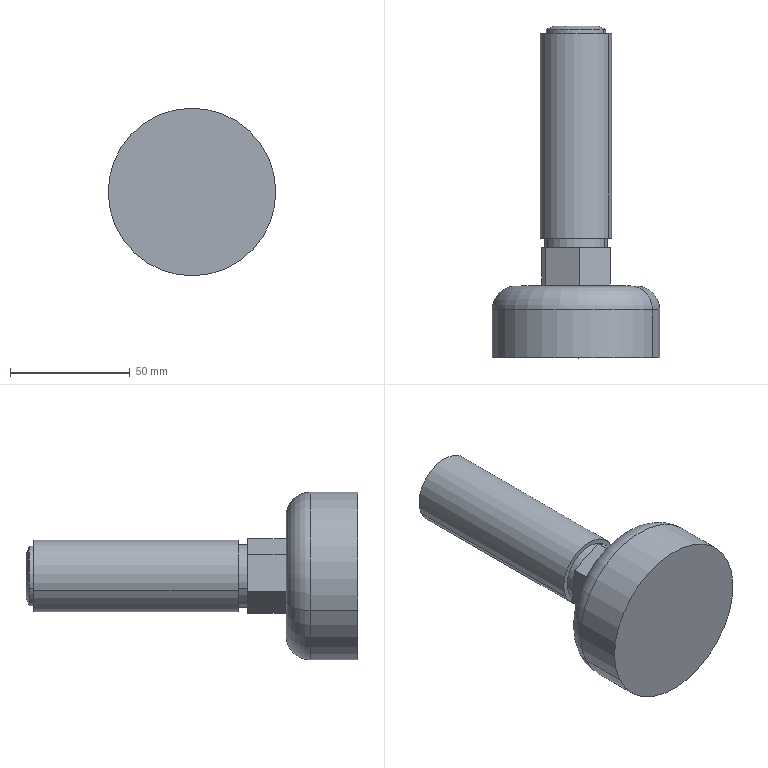Part | STEP file | Fillet 2-4 | 1 solid | 26 faces | box 70 x 138.618 x 70 mm | volume 157430 mm3 | plane 12 | cylinder 10 | torus 2 | sphere 2 | commonest cylinder face diameters 18 x2 25 x2 26 x2 30 x2 70 x2
STEP:
#1=CARTESIAN_POINT('',(-1171.526,-1356.736,3153.219));
#2=VERTEX_POINT('',#1);
#3=CARTESIAN_POINT('',(-1125.95,-1356.736,3173.781));
#4=VERTEX_POINT('',#3);
#5=CARTESIAN_POINT('',(-1148.738,-1356.736,3163.5));
#6=DIRECTION('',(0.,1.,0.));
#7=DIRECTION('',(0.9115,0.,0.4113));
#8=AXIS2_PLACEMENT_3D('',#5,#6,#7);
#9=CIRCLE('',#8,25.);
#10=EDGE_CURVE('',#2,#4,#9,.T.);
#11=ORIENTED_EDGE('',*,*,#10,.F.);
#12=CARTESIAN_POINT('',(-1180.641,-1366.736,3149.106));
#13=VERTEX_POINT('',#12);
#14=CARTESIAN_POINT('',(-1171.526,-1366.736,3153.219));
#15=DIRECTION('',(-0.4113,0.,0.9115));
#16=DIRECTION('',(-0.9115,0.,-0.4113));
#17=AXIS2_PLACEMENT_3D('',#14,#15,#16);
#18=CIRCLE('',#17,10.);
#19=EDGE_CURVE('',#2,#13,#18,.T.);
#20=ORIENTED_EDGE('',*,*,#19,.T.);
#21=CARTESIAN_POINT('',(-1116.835,-1366.736,3177.894));
#22=VERTEX_POINT('',#21);
#23=CARTESIAN_POINT('',(-1148.738,-1366.736,3163.5));
#24=DIRECTION('',(0.,-1.,0.));
#25=DIRECTION('',(0.9115,0.,0.4113));
#26=AXIS2_PLACEMENT_3D('',#23,#24,#25);
#27=CIRCLE('',#26,35.);
#28=EDGE_CURVE('',#22,#13,#27,.T.);
#29=ORIENTED_EDGE('',*,*,#28,.F.);
#30=CARTESIAN_POINT('',(-1125.95,-1366.736,3173.781));
#31=DIRECTION('',(0.4113,0.,-0.9115));
#32=DIRECTION('',(0.,1.,0.));
#33=AXIS2_PLACEMENT_3D('',#30,#31,#32);
#34=CIRCLE('',#33,10.);
#35=EDGE_CURVE('',#4,#22,#34,.T.);
#36=ORIENTED_EDGE('',*,*,#35,.F.);
#37=EDGE_LOOP('',(#11,#20,#29,#36));
#38=FACE_OUTER_BOUND('',#37,.T.);
#39=CARTESIAN_POINT('',(-1148.738,-1366.736,3163.5));
#40=DIRECTION('',(0.,-1.,0.));
#41=DIRECTION('',(-0.9115,0.,-0.4113));
#42=AXIS2_PLACEMENT_3D('',#39,#40,#41);
#43=TOROIDAL_SURFACE('',#42,25.,10.);
#44=ADVANCED_FACE('',(#38),#43,.T.);
#45=CARTESIAN_POINT('',(-1116.835,-1386.736,3177.894));
#46=VERTEX_POINT('',#45);
#47=CARTESIAN_POINT('',(-1180.641,-1386.736,3149.106));
#48=VERTEX_POINT('',#47);
#49=CARTESIAN_POINT('',(-1148.738,-1386.736,3163.5));
#50=DIRECTION('',(0.,-1.,0.));
#51=DIRECTION('',(0.9115,0.,0.4113));
#52=AXIS2_PLACEMENT_3D('',#49,#50,#51);
#53=CIRCLE('',#52,35.);
#54=EDGE_CURVE('',#46,#48,#53,.T.);
#55=ORIENTED_EDGE('',*,*,#54,.F.);
#56=CARTESIAN_POINT('',(-1116.835,-1386.736,3177.894));
#57=DIRECTION('',(0.,-1.,0.));
#58=VECTOR('',#57,1000.);
#59=LINE('',#56,#58);
#60=EDGE_CURVE('',#22,#46,#59,.T.);
#61=ORIENTED_EDGE('',*,*,#60,.F.);
#62=ORIENTED_EDGE('',*,*,#28,.T.);
#63=CARTESIAN_POINT('',(-1180.641,-1386.736,3149.106));
#64=DIRECTION('',(0.,-1.,0.));
#65=VECTOR('',#64,1000.);
#66=LINE('',#63,#65);
#67=EDGE_CURVE('',#13,#48,#66,.T.);
#68=ORIENTED_EDGE('',*,*,#67,.T.);
#69=EDGE_LOOP('',(#55,#61,#62,#68));
#70=FACE_OUTER_BOUND('',#69,.T.);
#71=CARTESIAN_POINT('',(-1148.738,-1386.736,3163.5));
#72=DIRECTION('',(0.,1.,0.));
#73=DIRECTION('',(0.9115,0.,0.4113));
#74=AXIS2_PLACEMENT_3D('',#71,#72,#73);
#75=CYLINDRICAL_SURFACE('',#74,35.);
#76=ADVANCED_FACE('',(#70),#75,.T.);
#77=CARTESIAN_POINT('',(-1160.132,-1251.236,3158.359));
#78=VERTEX_POINT('',#77);
#79=CARTESIAN_POINT('',(-1137.344,-1251.236,3168.641));
#80=VERTEX_POINT('',#79);
#81=CARTESIAN_POINT('',(-1148.738,-1251.236,3163.5));
#82=DIRECTION('',(0.,1.,0.));
#83=DIRECTION('',(-0.9115,0.,-0.4113));
#84=AXIS2_PLACEMENT_3D('',#81,#82,#83);
#85=CIRCLE('',#84,12.5);
#86=EDGE_CURVE('',#78,#80,#85,.T.);
#87=ORIENTED_EDGE('',*,*,#86,.T.);
#88=CARTESIAN_POINT('',(-1137.344,-1249.464,3168.641));
#89=VERTEX_POINT('',#88);
#90=CARTESIAN_POINT('',(-1137.344,-1246.736,3168.641));
#91=DIRECTION('',(0.,-1.,0.));
#92=VECTOR('',#91,1000.);
#93=LINE('',#90,#92);
#94=EDGE_CURVE('',#89,#80,#93,.T.);
#95=ORIENTED_EDGE('',*,*,#94,.F.);
#96=CARTESIAN_POINT('',(-1153.879,-1249.464,3174.894));
#97=VERTEX_POINT('',#96);
#98=CARTESIAN_POINT('',(-1148.738,-1249.464,3163.5));
#99=DIRECTION('',(0.,1.,0.));
#100=DIRECTION('',(-0.9115,0.,-0.4113));
#101=AXIS2_PLACEMENT_3D('',#98,#99,#100);
#102=CIRCLE('',#101,12.5);
#103=EDGE_CURVE('',#97,#89,#102,.T.);
#104=ORIENTED_EDGE('',*,*,#103,.F.);
#105=CARTESIAN_POINT('',(-1160.132,-1249.464,3158.359));
#106=VERTEX_POINT('',#105);
#107=CARTESIAN_POINT('',(-1148.738,-1249.464,3163.5));
#108=DIRECTION('',(0.,1.,0.));
#109=DIRECTION('',(-0.9115,0.,-0.4113));
#110=AXIS2_PLACEMENT_3D('',#107,#108,#109);
#111=CIRCLE('',#110,12.5);
#112=EDGE_CURVE('',#106,#97,#111,.T.);
#113=ORIENTED_EDGE('',*,*,#112,.F.);
#114=CARTESIAN_POINT('',(-1160.132,-1246.736,3158.359));
#115=DIRECTION('',(0.,-1.,0.));
#116=VECTOR('',#115,1000.);
#117=LINE('',#114,#116);
#118=EDGE_CURVE('',#106,#78,#117,.T.);
#119=ORIENTED_EDGE('',*,*,#118,.T.);
#120=EDGE_LOOP('',(#87,#95,#104,#113,#119));
#121=FACE_OUTER_BOUND('',#120,.T.);
#122=CARTESIAN_POINT('',(-1148.738,-1246.736,3163.5));
#123=DIRECTION('',(0.,1.,0.));
#124=DIRECTION('',(0.9115,0.,0.4113));
#125=AXIS2_PLACEMENT_3D('',#122,#123,#124);
#126=CYLINDRICAL_SURFACE('',#125,12.5);
#127=ADVANCED_FACE('',(#121),#126,.T.);
#128=ORIENTED_EDGE('',*,*,#103,.T.);
#129=CARTESIAN_POINT('',(-1143.598,-1249.464,3152.106));
#130=VERTEX_POINT('',#129);
#131=CARTESIAN_POINT('',(-1148.738,-1249.464,3163.5));
#132=DIRECTION('',(0.,1.,0.));
#133=DIRECTION('',(-0.9115,0.,-0.4113));
#134=AXIS2_PLACEMENT_3D('',#131,#132,#133);
#135=CIRCLE('',#134,12.5);
#136=EDGE_CURVE('',#89,#130,#135,.T.);
#137=ORIENTED_EDGE('',*,*,#136,.T.);
#138=CARTESIAN_POINT('',(-1145.037,-1248.118,3155.296));
#139=VERTEX_POINT('',#138);
#140=CARTESIAN_POINT('',(-1148.738,-1276.736,3163.5));
#141=DIRECTION('',(0.9115,0.,0.4113));
#142=DIRECTION('',(-0.4113,0.,0.9115));
#143=AXIS2_PLACEMENT_3D('',#140,#141,#142);
#144=CIRCLE('',#143,30.);
#145=EDGE_CURVE('',#130,#139,#144,.T.);
#146=ORIENTED_EDGE('',*,*,#145,.T.);
#147=CARTESIAN_POINT('',(-1140.535,-1248.118,3167.201));
#148=VERTEX_POINT('',#147);
#149=CARTESIAN_POINT('',(-1148.738,-1248.118,3163.5));
#150=DIRECTION('',(0.,1.,0.));
#151=DIRECTION('',(0.9115,0.,0.4113));
#152=AXIS2_PLACEMENT_3D('',#149,#150,#151);
#153=CIRCLE('',#152,9.);
#154=EDGE_CURVE('',#148,#139,#153,.T.);
#155=ORIENTED_EDGE('',*,*,#154,.F.);
#156=CARTESIAN_POINT('',(-1152.44,-1248.118,3171.704));
#157=VERTEX_POINT('',#156);
#158=CARTESIAN_POINT('',(-1148.738,-1248.118,3163.5));
#159=DIRECTION('',(0.,1.,0.));
#160=DIRECTION('',(0.9115,0.,0.4113));
#161=AXIS2_PLACEMENT_3D('',#158,#159,#160);
#162=CIRCLE('',#161,9.);
#163=EDGE_CURVE('',#157,#148,#162,.T.);
#164=ORIENTED_EDGE('',*,*,#163,.F.);
#165=CARTESIAN_POINT('',(-1148.738,-1276.736,3163.5));
#166=DIRECTION('',(-0.9115,0.,-0.4113));
#167=DIRECTION('',(0.,-1.,0.));
#168=AXIS2_PLACEMENT_3D('',#165,#166,#167);
#169=CIRCLE('',#168,30.);
#170=EDGE_CURVE('',#97,#157,#169,.T.);
#171=ORIENTED_EDGE('',*,*,#170,.F.);
#172=EDGE_LOOP('',(#128,#137,#146,#155,#164,#171));
#173=FACE_OUTER_BOUND('',#172,.T.);
#174=CARTESIAN_POINT('',(-1148.738,-1276.736,3163.5));
#175=DIRECTION('',(0.,1.,0.));
#176=DIRECTION('',(0.4113,0.,-0.9115));
#177=AXIS2_PLACEMENT_3D('',#174,#175,#176);
#178=SPHERICAL_SURFACE('',#177,30.);
#179=ADVANCED_FACE('',(#173),#178,.T.);
#180=ORIENTED_EDGE('',*,*,#154,.T.);
#181=CARTESIAN_POINT('',(-1156.942,-1248.118,3159.799));
#182=VERTEX_POINT('',#181);
#183=CARTESIAN_POINT('',(-1148.738,-1248.118,3163.5));
#184=DIRECTION('',(0.,1.,0.));
#185=DIRECTION('',(0.9115,0.,0.4113));
#186=AXIS2_PLACEMENT_3D('',#183,#184,#185);
#187=CIRCLE('',#186,9.);
#188=EDGE_CURVE('',#139,#182,#187,.T.);
#189=ORIENTED_EDGE('',*,*,#188,.T.);
#190=CARTESIAN_POINT('',(-1156.942,-1356.736,3159.799));
#191=VERTEX_POINT('',#190);
#192=CARTESIAN_POINT('',(-1156.942,-1246.735,3159.799));
#193=DIRECTION('',(0.,-1.,0.));
#194=VECTOR('',#193,1000.);
#195=LINE('',#192,#194);
#196=EDGE_CURVE('',#182,#191,#195,.T.);
#197=ORIENTED_EDGE('',*,*,#196,.T.);
#198=CARTESIAN_POINT('',(-1140.535,-1356.736,3167.201));
#199=VERTEX_POINT('',#198);
#200=CARTESIAN_POINT('',(-1148.738,-1356.736,3163.5));
#201=DIRECTION('',(0.,-1.,0.));
#202=DIRECTION('',(0.9115,0.,0.4113));
#203=AXIS2_PLACEMENT_3D('',#200,#201,#202);
#204=CIRCLE('',#203,9.);
#205=EDGE_CURVE('',#191,#199,#204,.T.);
#206=ORIENTED_EDGE('',*,*,#205,.T.);
#207=CARTESIAN_POINT('',(-1140.535,-1246.735,3167.201));
#208=DIRECTION('',(0.,-1.,0.));
#209=VECTOR('',#208,1000.);
#210=LINE('',#207,#209);
#211=EDGE_CURVE('',#148,#199,#210,.T.);
#212=ORIENTED_EDGE('',*,*,#211,.F.);
#213=EDGE_LOOP('',(#180,#189,#197,#206,#212));
#214=FACE_OUTER_BOUND('',#213,.T.);
#215=CARTESIAN_POINT('',(-1148.738,-1246.735,3163.5));
#216=DIRECTION('',(0.,-1.,0.));
#217=DIRECTION('',(-0.9115,0.,-0.4113));
#218=AXIS2_PLACEMENT_3D('',#215,#216,#217);
#219=CYLINDRICAL_SURFACE('',#218,9.);
#220=ADVANCED_FACE('',(#214),#219,.F.);
#221=CARTESIAN_POINT('',(-1136.889,-1340.736,3168.846));
#222=VERTEX_POINT('',#221);
#223=CARTESIAN_POINT('',(-1160.588,-1340.736,3158.154));
#224=VERTEX_POINT('',#223);
#225=CARTESIAN_POINT('',(-1148.738,-1340.736,3163.5));
#226=DIRECTION('',(0.,-1.,0.));
#227=DIRECTION('',(0.9115,0.,0.4113));
#228=AXIS2_PLACEMENT_3D('',#225,#226,#227);
#229=CIRCLE('',#228,13.);
#230=EDGE_CURVE('',#222,#224,#229,.T.);
#231=ORIENTED_EDGE('',*,*,#230,.F.);
#232=CARTESIAN_POINT('',(-1136.889,-1336.736,3168.846));
#233=VERTEX_POINT('',#232);
#234=CARTESIAN_POINT('',(-1136.889,-1340.736,3168.846));
#235=DIRECTION('',(0.,-1.,0.));
#236=VECTOR('',#235,1000.);
#237=LINE('',#234,#236);
#238=EDGE_CURVE('',#233,#222,#237,.T.);
#239=ORIENTED_EDGE('',*,*,#238,.F.);
#240=CARTESIAN_POINT('',(-1160.588,-1336.736,3158.154));
#241=VERTEX_POINT('',#240);
#242=CARTESIAN_POINT('',(-1148.738,-1336.736,3163.5));
#243=DIRECTION('',(0.,-1.,0.));
#244=DIRECTION('',(0.9115,0.,0.4113));
#245=AXIS2_PLACEMENT_3D('',#242,#243,#244);
#246=CIRCLE('',#245,13.);
#247=EDGE_CURVE('',#233,#241,#246,.T.);
#248=ORIENTED_EDGE('',*,*,#247,.T.);
#249=CARTESIAN_POINT('',(-1160.588,-1340.736,3158.154));
#250=DIRECTION('',(0.,-1.,0.));
#251=VECTOR('',#250,1000.);
#252=LINE('',#249,#251);
#253=EDGE_CURVE('',#241,#224,#252,.T.);
#254=ORIENTED_EDGE('',*,*,#253,.T.);
#255=EDGE_LOOP('',(#231,#239,#248,#254));
#256=FACE_OUTER_BOUND('',#255,.T.);
#257=CARTESIAN_POINT('',(-1148.738,-1340.736,3163.5));
#258=DIRECTION('',(0.,1.,0.));
#259=DIRECTION('',(0.9115,0.,0.4113));
#260=AXIS2_PLACEMENT_3D('',#257,#258,#259);
#261=CYLINDRICAL_SURFACE('',#260,13.);
#262=ADVANCED_FACE('',(#256),#261,.T.);
#263=CARTESIAN_POINT('',(-1135.065,-1336.736,3169.669));
#264=VERTEX_POINT('',#263);
#265=CARTESIAN_POINT('',(-1162.411,-1336.736,3157.331));
#266=VERTEX_POINT('',#265);
#267=CARTESIAN_POINT('',(-1148.738,-1336.736,3163.5));
#268=DIRECTION('',(0.,-1.,0.));
#269=DIRECTION('',(0.9115,0.,0.4113));
#270=AXIS2_PLACEMENT_3D('',#267,#268,#269);
#271=CIRCLE('',#270,15.);
#272=EDGE_CURVE('',#264,#266,#271,.T.);
#273=ORIENTED_EDGE('',*,*,#272,.F.);
#274=CARTESIAN_POINT('',(-1135.065,-1251.236,3169.669));
#275=VERTEX_POINT('',#274);
#276=CARTESIAN_POINT('',(-1135.065,-1336.736,3169.669));
#277=DIRECTION('',(0.,-1.,0.));
#278=VECTOR('',#277,1000.);
#279=LINE('',#276,#278);
#280=EDGE_CURVE('',#275,#264,#279,.T.);
#281=ORIENTED_EDGE('',*,*,#280,.F.);
#282=CARTESIAN_POINT('',(-1162.411,-1251.236,3157.331));
#283=VERTEX_POINT('',#282);
#284=CARTESIAN_POINT('',(-1148.738,-1251.236,3163.5));
#285=DIRECTION('',(0.,1.,0.));
#286=DIRECTION('',(-0.9115,0.,-0.4113));
#287=AXIS2_PLACEMENT_3D('',#284,#285,#286);
#288=CIRCLE('',#287,15.);
#289=EDGE_CURVE('',#283,#275,#288,.T.);
#290=ORIENTED_EDGE('',*,*,#289,.F.);
#291=CARTESIAN_POINT('',(-1162.411,-1336.736,3157.331));
#292=DIRECTION('',(0.,-1.,0.));
#293=VECTOR('',#292,1000.);
#294=LINE('',#291,#293);
#295=EDGE_CURVE('',#283,#266,#294,.T.);
#296=ORIENTED_EDGE('',*,*,#295,.T.);
#297=EDGE_LOOP('',(#273,#281,#290,#296));
#298=FACE_OUTER_BOUND('',#297,.T.);
#299=CARTESIAN_POINT('',(-1148.738,-1336.736,3163.5));
#300=DIRECTION('',(0.,1.,0.));
#301=DIRECTION('',(0.9115,0.,0.4113));
#302=AXIS2_PLACEMENT_3D('',#299,#300,#301);
#303=CYLINDRICAL_SURFACE('',#302,15.);
#304=ADVANCED_FACE('',(#298),#303,.T.);
#305=CARTESIAN_POINT('',(-1148.738,-1336.736,3163.5));
#306=DIRECTION('',(0.,-1.,0.));
#307=DIRECTION('',(0.9115,0.,0.4113));
#308=AXIS2_PLACEMENT_3D('',#305,#306,#307);
#309=CIRCLE('',#308,15.);
#310=EDGE_CURVE('',#266,#264,#309,.T.);
#311=ORIENTED_EDGE('',*,*,#310,.T.);
#312=ORIENTED_EDGE('',*,*,#272,.T.);
#313=EDGE_LOOP('',(#311,#312));
#314=FACE_OUTER_BOUND('',#313,.T.);
#315=CARTESIAN_POINT('',(-1148.738,-1336.736,3163.5));
#316=DIRECTION('',(0.,-1.,0.));
#317=DIRECTION('',(0.9115,0.,0.4113));
#318=AXIS2_PLACEMENT_3D('',#315,#316,#317);
#319=CIRCLE('',#318,13.);
#320=EDGE_CURVE('',#241,#233,#319,.T.);
#321=ORIENTED_EDGE('',*,*,#320,.F.);
#322=ORIENTED_EDGE('',*,*,#247,.F.);
#323=EDGE_LOOP('',(#321,#322));
#324=FACE_BOUND('',#323,.T.);
#325=CARTESIAN_POINT('',(-1148.738,-1336.736,3163.5));
#326=DIRECTION('',(0.,-1.,0.));
#327=DIRECTION('',(-0.9115,0.,-0.4113));
#328=AXIS2_PLACEMENT_3D('',#325,#326,#327);
#329=PLANE('',#328);
#330=ADVANCED_FACE('',(#314,#324),#329,.T.);
#331=ORIENTED_EDGE('',*,*,#280,.T.);
#332=ORIENTED_EDGE('',*,*,#310,.F.);
#333=ORIENTED_EDGE('',*,*,#295,.F.);
#334=CARTESIAN_POINT('',(-1148.738,-1251.236,3163.5));
#335=DIRECTION('',(0.,1.,0.));
#336=DIRECTION('',(-0.9115,0.,-0.4113));
#337=AXIS2_PLACEMENT_3D('',#334,#335,#336);
#338=CIRCLE('',#337,15.);
#339=EDGE_CURVE('',#275,#283,#338,.T.);
#340=ORIENTED_EDGE('',*,*,#339,.F.);
#341=EDGE_LOOP('',(#331,#332,#333,#340));
#342=FACE_OUTER_BOUND('',#341,.T.);
#343=CARTESIAN_POINT('',(-1148.738,-1336.736,3163.5));
#344=DIRECTION('',(0.,1.,0.));
#345=DIRECTION('',(0.9115,0.,0.4113));
#346=AXIS2_PLACEMENT_3D('',#343,#344,#345);
#347=CYLINDRICAL_SURFACE('',#346,15.);
#348=ADVANCED_FACE('',(#342),#347,.T.);
#349=ORIENTED_EDGE('',*,*,#238,.T.);
#350=CARTESIAN_POINT('',(-1148.738,-1340.736,3163.5));
#351=DIRECTION('',(0.,-1.,0.));
#352=DIRECTION('',(0.9115,0.,0.4113));
#353=AXIS2_PLACEMENT_3D('',#350,#351,#352);
#354=CIRCLE('',#353,13.);
#355=EDGE_CURVE('',#224,#222,#354,.T.);
#356=ORIENTED_EDGE('',*,*,#355,.F.);
#357=ORIENTED_EDGE('',*,*,#253,.F.);
#358=ORIENTED_EDGE('',*,*,#320,.T.);
#359=EDGE_LOOP('',(#349,#356,#357,#358));
#360=FACE_OUTER_BOUND('',#359,.T.);
#361=CARTESIAN_POINT('',(-1148.738,-1340.736,3163.5));
#362=DIRECTION('',(0.,1.,0.));
#363=DIRECTION('',(0.9115,0.,0.4113));
#364=AXIS2_PLACEMENT_3D('',#361,#362,#363);
#365=CYLINDRICAL_SURFACE('',#364,13.);
#366=ADVANCED_FACE('',(#360),#365,.T.);
#367=CARTESIAN_POINT('',(-1136.082,-1340.736,3154.4));
#368=VERTEX_POINT('',#367);
#369=CARTESIAN_POINT('',(-1134.529,-1340.736,3169.911));
#370=VERTEX_POINT('',#369);
#371=CARTESIAN_POINT('',(-1136.082,-1340.736,3154.4));
#372=DIRECTION('',(0.0996,0.,0.995));
#373=VECTOR('',#372,1000.);
#374=LINE('',#371,#373);
#375=EDGE_CURVE('',#368,#370,#374,.T.);
#376=ORIENTED_EDGE('',*,*,#375,.F.);
#377=CARTESIAN_POINT('',(-1150.291,-1340.736,3147.989));
#378=VERTEX_POINT('',#377);
#379=CARTESIAN_POINT('',(-1150.291,-1340.736,3147.989));
#380=DIRECTION('',(0.9115,0.,0.4113));
#381=VECTOR('',#380,1000.);
#382=LINE('',#379,#381);
#383=EDGE_CURVE('',#378,#368,#382,.T.);
#384=ORIENTED_EDGE('',*,*,#383,.F.);
#385=CARTESIAN_POINT('',(-1162.947,-1340.736,3157.089));
#386=VERTEX_POINT('',#385);
#387=CARTESIAN_POINT('',(-1162.947,-1340.736,3157.089));
#388=DIRECTION('',(0.8119,0.,-0.5838));
#389=VECTOR('',#388,1000.);
#390=LINE('',#387,#389);
#391=EDGE_CURVE('',#386,#378,#390,.T.);
#392=ORIENTED_EDGE('',*,*,#391,.F.);
#393=CARTESIAN_POINT('',(-1161.395,-1340.736,3172.6));
#394=VERTEX_POINT('',#393);
#395=CARTESIAN_POINT('',(-1161.395,-1340.736,3172.6));
#396=DIRECTION('',(-0.0996,0.,-0.995));
#397=VECTOR('',#396,1000.);
#398=LINE('',#395,#397);
#399=EDGE_CURVE('',#394,#386,#398,.T.);
#400=ORIENTED_EDGE('',*,*,#399,.F.);
#401=CARTESIAN_POINT('',(-1147.186,-1340.736,3179.011));
#402=VERTEX_POINT('',#401);
#403=CARTESIAN_POINT('',(-1147.186,-1340.736,3179.011));
#404=DIRECTION('',(-0.9115,0.,-0.4113));
#405=VECTOR('',#404,1000.);
#406=LINE('',#403,#405);
#407=EDGE_CURVE('',#402,#394,#406,.T.);
#408=ORIENTED_EDGE('',*,*,#407,.F.);
#409=CARTESIAN_POINT('',(-1134.529,-1340.736,3169.911));
#410=DIRECTION('',(-0.8119,0.,0.5838));
#411=VECTOR('',#410,1000.);
#412=LINE('',#409,#411);
#413=EDGE_CURVE('',#370,#402,#412,.T.);
#414=ORIENTED_EDGE('',*,*,#413,.F.);
#415=EDGE_LOOP('',(#376,#384,#392,#400,#408,#414));
#416=FACE_OUTER_BOUND('',#415,.T.);
#417=ORIENTED_EDGE('',*,*,#355,.T.);
#418=ORIENTED_EDGE('',*,*,#230,.T.);
#419=EDGE_LOOP('',(#417,#418));
#420=FACE_BOUND('',#419,.T.);
#421=CARTESIAN_POINT('',(-1148.738,-1340.736,3163.5));
#422=DIRECTION('',(0.,-1.,0.));
#423=DIRECTION('',(-0.9115,0.,-0.4113));
#424=AXIS2_PLACEMENT_3D('',#421,#422,#423);
#425=PLANE('',#424);
#426=ADVANCED_FACE('',(#416,#420),#425,.F.);
#427=ORIENTED_EDGE('',*,*,#375,.T.);
#428=CARTESIAN_POINT('',(-1134.529,-1356.736,3169.911));
#429=VERTEX_POINT('',#428);
#430=CARTESIAN_POINT('',(-1134.529,-1356.736,3169.911));
#431=DIRECTION('',(0.,1.,0.));
#432=VECTOR('',#431,1000.);
#433=LINE('',#430,#432);
#434=EDGE_CURVE('',#429,#370,#433,.T.);
#435=ORIENTED_EDGE('',*,*,#434,.F.);
#436=CARTESIAN_POINT('',(-1136.082,-1356.736,3154.4));
#437=VERTEX_POINT('',#436);
#438=CARTESIAN_POINT('',(-1136.082,-1356.736,3154.4));
#439=DIRECTION('',(0.0996,0.,0.995));
#440=VECTOR('',#439,1000.);
#441=LINE('',#438,#440);
#442=EDGE_CURVE('',#437,#429,#441,.T.);
#443=ORIENTED_EDGE('',*,*,#442,.F.);
#444=CARTESIAN_POINT('',(-1136.082,-1356.736,3154.4));
#445=DIRECTION('',(0.,1.,0.));
#446=VECTOR('',#445,1000.);
#447=LINE('',#444,#446);
#448=EDGE_CURVE('',#437,#368,#447,.T.);
#449=ORIENTED_EDGE('',*,*,#448,.T.);
#450=EDGE_LOOP('',(#427,#435,#443,#449));
#451=FACE_OUTER_BOUND('',#450,.T.);
#452=CARTESIAN_POINT('',(-1136.082,-1356.736,3154.4));
#453=DIRECTION('',(-0.995,0.,0.0996));
#454=DIRECTION('',(0.0996,0.,0.995));
#455=AXIS2_PLACEMENT_3D('',#452,#453,#454);
#456=PLANE('',#455);
#457=ADVANCED_FACE('',(#451),#456,.F.);
#458=ORIENTED_EDGE('',*,*,#413,.T.);
#459=CARTESIAN_POINT('',(-1147.186,-1356.736,3179.011));
#460=VERTEX_POINT('',#459);
#461=CARTESIAN_POINT('',(-1147.186,-1356.736,3179.011));
#462=DIRECTION('',(0.,1.,0.));
#463=VECTOR('',#462,1000.);
#464=LINE('',#461,#463);
#465=EDGE_CURVE('',#460,#402,#464,.T.);
#466=ORIENTED_EDGE('',*,*,#465,.F.);
#467=CARTESIAN_POINT('',(-1134.529,-1356.736,3169.911));
#468=DIRECTION('',(-0.8119,0.,0.5838));
#469=VECTOR('',#468,1000.);
#470=LINE('',#467,#469);
#471=EDGE_CURVE('',#429,#460,#470,.T.);
#472=ORIENTED_EDGE('',*,*,#471,.F.);
#473=ORIENTED_EDGE('',*,*,#434,.T.);
#474=EDGE_LOOP('',(#458,#466,#472,#473));
#475=FACE_OUTER_BOUND('',#474,.T.);
#476=CARTESIAN_POINT('',(-1134.529,-1356.736,3169.911));
#477=DIRECTION('',(-0.5838,0.,-0.8119));
#478=DIRECTION('',(-0.8119,0.,0.5838));
#479=AXIS2_PLACEMENT_3D('',#476,#477,#478);
#480=PLANE('',#479);
#481=ADVANCED_FACE('',(#475),#480,.F.);
#482=ORIENTED_EDGE('',*,*,#407,.T.);
#483=CARTESIAN_POINT('',(-1161.395,-1356.736,3172.6));
#484=VERTEX_POINT('',#483);
#485=CARTESIAN_POINT('',(-1161.395,-1356.736,3172.6));
#486=DIRECTION('',(0.,1.,0.));
#487=VECTOR('',#486,1000.);
#488=LINE('',#485,#487);
#489=EDGE_CURVE('',#484,#394,#488,.T.);
#490=ORIENTED_EDGE('',*,*,#489,.F.);
#491=CARTESIAN_POINT('',(-1147.186,-1356.736,3179.011));
#492=DIRECTION('',(-0.9115,0.,-0.4113));
#493=VECTOR('',#492,1000.);
#494=LINE('',#491,#493);
#495=EDGE_CURVE('',#460,#484,#494,.T.);
#496=ORIENTED_EDGE('',*,*,#495,.F.);
#497=ORIENTED_EDGE('',*,*,#465,.T.);
#498=EDGE_LOOP('',(#482,#490,#496,#497));
#499=FACE_OUTER_BOUND('',#498,.T.);
#500=CARTESIAN_POINT('',(-1147.186,-1356.736,3179.011));
#501=DIRECTION('',(0.4113,0.,-0.9115));
#502=DIRECTION('',(-0.9115,0.,-0.4113));
#503=AXIS2_PLACEMENT_3D('',#500,#501,#502);
#504=PLANE('',#503);
#505=ADVANCED_FACE('',(#499),#504,.F.);
#506=ORIENTED_EDGE('',*,*,#399,.T.);
#507=CARTESIAN_POINT('',(-1162.947,-1356.736,3157.089));
#508=VERTEX_POINT('',#507);
#509=CARTESIAN_POINT('',(-1162.947,-1356.736,3157.089));
#510=DIRECTION('',(0.,1.,0.));
#511=VECTOR('',#510,1000.);
#512=LINE('',#509,#511);
#513=EDGE_CURVE('',#508,#386,#512,.T.);
#514=ORIENTED_EDGE('',*,*,#513,.F.);
#515=CARTESIAN_POINT('',(-1161.395,-1356.736,3172.6));
#516=DIRECTION('',(-0.0996,0.,-0.995));
#517=VECTOR('',#516,1000.);
#518=LINE('',#515,#517);
#519=EDGE_CURVE('',#484,#508,#518,.T.);
#520=ORIENTED_EDGE('',*,*,#519,.F.);
#521=ORIENTED_EDGE('',*,*,#489,.T.);
#522=EDGE_LOOP('',(#506,#514,#520,#521));
#523=FACE_OUTER_BOUND('',#522,.T.);
#524=CARTESIAN_POINT('',(-1161.395,-1356.736,3172.6));
#525=DIRECTION('',(0.995,0.,-0.0996));
#526=DIRECTION('',(-0.0996,0.,-0.995));
#527=AXIS2_PLACEMENT_3D('',#524,#525,#526);
#528=PLANE('',#527);
#529=ADVANCED_FACE('',(#523),#528,.F.);
#530=ORIENTED_EDGE('',*,*,#391,.T.);
#531=CARTESIAN_POINT('',(-1150.291,-1356.736,3147.989));
#532=VERTEX_POINT('',#531);
#533=CARTESIAN_POINT('',(-1150.291,-1356.736,3147.989));
#534=DIRECTION('',(0.,1.,0.));
#535=VECTOR('',#534,1000.);
#536=LINE('',#533,#535);
#537=EDGE_CURVE('',#532,#378,#536,.T.);
#538=ORIENTED_EDGE('',*,*,#537,.F.);
#539=CARTESIAN_POINT('',(-1162.947,-1356.736,3157.089));
#540=DIRECTION('',(0.8119,0.,-0.5838));
#541=VECTOR('',#540,1000.);
#542=LINE('',#539,#541);
#543=EDGE_CURVE('',#508,#532,#542,.T.);
#544=ORIENTED_EDGE('',*,*,#543,.F.);
#545=ORIENTED_EDGE('',*,*,#513,.T.);
#546=EDGE_LOOP('',(#530,#538,#544,#545));
#547=FACE_OUTER_BOUND('',#546,.T.);
#548=CARTESIAN_POINT('',(-1162.947,-1356.736,3157.089));
#549=DIRECTION('',(0.5838,0.,0.8119));
#550=DIRECTION('',(0.8119,0.,-0.5838));
#551=AXIS2_PLACEMENT_3D('',#548,#549,#550);
#552=PLANE('',#551);
#553=ADVANCED_FACE('',(#547),#552,.F.);
#554=ORIENTED_EDGE('',*,*,#383,.T.);
#555=ORIENTED_EDGE('',*,*,#448,.F.);
#556=CARTESIAN_POINT('',(-1150.291,-1356.736,3147.989));
#557=DIRECTION('',(0.9115,0.,0.4113));
#558=VECTOR('',#557,1000.);
#559=LINE('',#556,#558);
#560=EDGE_CURVE('',#532,#437,#559,.T.);
#561=ORIENTED_EDGE('',*,*,#560,.F.);
#562=ORIENTED_EDGE('',*,*,#537,.T.);
#563=EDGE_LOOP('',(#554,#555,#561,#562));
#564=FACE_OUTER_BOUND('',#563,.T.);
#565=CARTESIAN_POINT('',(-1150.291,-1356.736,3147.989));
#566=DIRECTION('',(-0.4113,0.,0.9115));
#567=DIRECTION('',(0.9115,0.,0.4113));
#568=AXIS2_PLACEMENT_3D('',#565,#566,#567);
#569=PLANE('',#568);
#570=ADVANCED_FACE('',(#564),#569,.F.);
#571=ORIENTED_EDGE('',*,*,#196,.F.);
#572=CARTESIAN_POINT('',(-1148.738,-1248.118,3163.5));
#573=DIRECTION('',(0.,1.,0.));
#574=DIRECTION('',(0.9115,0.,0.4113));
#575=AXIS2_PLACEMENT_3D('',#572,#573,#574);
#576=CIRCLE('',#575,9.);
#577=EDGE_CURVE('',#182,#157,#576,.T.);
#578=ORIENTED_EDGE('',*,*,#577,.T.);
#579=ORIENTED_EDGE('',*,*,#163,.T.);
#580=ORIENTED_EDGE('',*,*,#211,.T.);
#581=CARTESIAN_POINT('',(-1148.738,-1356.736,3163.5));
#582=DIRECTION('',(0.,-1.,0.));
#583=DIRECTION('',(0.9115,0.,0.4113));
#584=AXIS2_PLACEMENT_3D('',#581,#582,#583);
#585=CIRCLE('',#584,9.);
#586=EDGE_CURVE('',#199,#191,#585,.T.);
#587=ORIENTED_EDGE('',*,*,#586,.T.);
#588=EDGE_LOOP('',(#571,#578,#579,#580,#587));
#589=FACE_OUTER_BOUND('',#588,.T.);
#590=CARTESIAN_POINT('',(-1148.738,-1246.735,3163.5));
#591=DIRECTION('',(0.,-1.,0.));
#592=DIRECTION('',(-0.9115,0.,-0.4113));
#593=AXIS2_PLACEMENT_3D('',#590,#591,#592);
#594=CYLINDRICAL_SURFACE('',#593,9.);
#595=ADVANCED_FACE('',(#589),#594,.F.);
#596=ORIENTED_EDGE('',*,*,#145,.F.);
#597=CARTESIAN_POINT('',(-1148.738,-1249.464,3163.5));
#598=DIRECTION('',(0.,1.,0.));
#599=DIRECTION('',(-0.9115,0.,-0.4113));
#600=AXIS2_PLACEMENT_3D('',#597,#598,#599);
#601=CIRCLE('',#600,12.5);
#602=EDGE_CURVE('',#130,#106,#601,.T.);
#603=ORIENTED_EDGE('',*,*,#602,.T.);
#604=ORIENTED_EDGE('',*,*,#112,.T.);
#605=ORIENTED_EDGE('',*,*,#170,.T.);
#606=ORIENTED_EDGE('',*,*,#577,.F.);
#607=ORIENTED_EDGE('',*,*,#188,.F.);
#608=EDGE_LOOP('',(#596,#603,#604,#605,#606,#607));
#609=FACE_OUTER_BOUND('',#608,.T.);
#610=CARTESIAN_POINT('',(-1148.738,-1276.736,3163.5));
#611=DIRECTION('',(0.,1.,0.));
#612=DIRECTION('',(0.4113,0.,-0.9115));
#613=AXIS2_PLACEMENT_3D('',#610,#611,#612);
#614=SPHERICAL_SURFACE('',#613,30.);
#615=ADVANCED_FACE('',(#609),#614,.T.);
#616=ORIENTED_EDGE('',*,*,#86,.F.);
#617=CARTESIAN_POINT('',(-1148.738,-1251.236,3163.5));
#618=DIRECTION('',(0.,1.,0.));
#619=DIRECTION('',(-0.9115,0.,-0.4113));
#620=AXIS2_PLACEMENT_3D('',#617,#618,#619);
#621=CIRCLE('',#620,12.5);
#622=EDGE_CURVE('',#80,#78,#621,.T.);
#623=ORIENTED_EDGE('',*,*,#622,.F.);
#624=EDGE_LOOP('',(#616,#623));
#625=FACE_BOUND('',#624,.T.);
#626=ORIENTED_EDGE('',*,*,#289,.T.);
#627=ORIENTED_EDGE('',*,*,#339,.T.);
#628=EDGE_LOOP('',(#626,#627));
#629=FACE_OUTER_BOUND('',#628,.T.);
#630=CARTESIAN_POINT('',(-1153.879,-1251.236,3174.894));
#631=DIRECTION('',(0.,-1.,0.));
#632=DIRECTION('',(-0.9115,0.,-0.4113));
#633=AXIS2_PLACEMENT_3D('',#630,#631,#632);
#634=PLANE('',#633);
#635=ADVANCED_FACE('',(#625,#629),#634,.F.);
#636=ORIENTED_EDGE('',*,*,#94,.T.);
#637=ORIENTED_EDGE('',*,*,#622,.T.);
#638=ORIENTED_EDGE('',*,*,#118,.F.);
#639=ORIENTED_EDGE('',*,*,#602,.F.);
#640=ORIENTED_EDGE('',*,*,#136,.F.);
#641=EDGE_LOOP('',(#636,#637,#638,#639,#640));
#642=FACE_OUTER_BOUND('',#641,.T.);
#643=CARTESIAN_POINT('',(-1148.738,-1246.736,3163.5));
#644=DIRECTION('',(0.,1.,0.));
#645=DIRECTION('',(0.9115,0.,0.4113));
#646=AXIS2_PLACEMENT_3D('',#643,#644,#645);
#647=CYLINDRICAL_SURFACE('',#646,12.5);
#648=ADVANCED_FACE('',(#642),#647,.T.);
#649=CARTESIAN_POINT('',(-1148.738,-1386.736,3163.5));
#650=DIRECTION('',(0.,-1.,0.));
#651=DIRECTION('',(0.9115,0.,0.4113));
#652=AXIS2_PLACEMENT_3D('',#649,#650,#651);
#653=CIRCLE('',#652,35.);
#654=EDGE_CURVE('',#48,#46,#653,.T.);
#655=ORIENTED_EDGE('',*,*,#654,.T.);
#656=ORIENTED_EDGE('',*,*,#54,.T.);
#657=EDGE_LOOP('',(#655,#656));
#658=FACE_OUTER_BOUND('',#657,.T.);
#659=CARTESIAN_POINT('',(-1148.738,-1386.736,3163.5));
#660=DIRECTION('',(0.,-1.,0.));
#661=DIRECTION('',(-0.9115,0.,-0.4113));
#662=AXIS2_PLACEMENT_3D('',#659,#660,#661);
#663=PLANE('',#662);
#664=ADVANCED_FACE('',(#658),#663,.T.);
#665=ORIENTED_EDGE('',*,*,#60,.T.);
#666=ORIENTED_EDGE('',*,*,#654,.F.);
#667=ORIENTED_EDGE('',*,*,#67,.F.);
#668=CARTESIAN_POINT('',(-1148.738,-1366.736,3163.5));
#669=DIRECTION('',(0.,-1.,0.));
#670=DIRECTION('',(0.9115,0.,0.4113));
#671=AXIS2_PLACEMENT_3D('',#668,#669,#670);
#672=CIRCLE('',#671,35.);
#673=EDGE_CURVE('',#13,#22,#672,.T.);
#674=ORIENTED_EDGE('',*,*,#673,.T.);
#675=EDGE_LOOP('',(#665,#666,#667,#674));
#676=FACE_OUTER_BOUND('',#675,.T.);
#677=CARTESIAN_POINT('',(-1148.738,-1386.736,3163.5));
#678=DIRECTION('',(0.,1.,0.));
#679=DIRECTION('',(0.9115,0.,0.4113));
#680=AXIS2_PLACEMENT_3D('',#677,#678,#679);
#681=CYLINDRICAL_SURFACE('',#680,35.);
#682=ADVANCED_FACE('',(#676),#681,.T.);
#683=CARTESIAN_POINT('',(-1148.738,-1356.736,3163.5));
#684=DIRECTION('',(0.,1.,0.));
#685=DIRECTION('',(0.9115,0.,0.4113));
#686=AXIS2_PLACEMENT_3D('',#683,#684,#685);
#687=CIRCLE('',#686,25.);
#688=EDGE_CURVE('',#4,#2,#687,.T.);
#689=ORIENTED_EDGE('',*,*,#688,.T.);
#690=ORIENTED_EDGE('',*,*,#10,.T.);
#691=EDGE_LOOP('',(#689,#690));
#692=FACE_OUTER_BOUND('',#691,.T.);
#693=ORIENTED_EDGE('',*,*,#560,.T.);
#694=ORIENTED_EDGE('',*,*,#442,.T.);
#695=ORIENTED_EDGE('',*,*,#471,.T.);
#696=ORIENTED_EDGE('',*,*,#495,.T.);
#697=ORIENTED_EDGE('',*,*,#519,.T.);
#698=ORIENTED_EDGE('',*,*,#543,.T.);
#699=EDGE_LOOP('',(#693,#694,#695,#696,#697,#698));
#700=FACE_BOUND('',#699,.T.);
#701=CARTESIAN_POINT('',(-1148.738,-1356.736,3163.5));
#702=DIRECTION('',(0.,-1.,0.));
#703=DIRECTION('',(-0.9115,0.,-0.4113));
#704=AXIS2_PLACEMENT_3D('',#701,#702,#703);
#705=PLANE('',#704);
#706=ADVANCED_FACE('',(#692,#700),#705,.F.);
#707=ORIENTED_EDGE('',*,*,#586,.F.);
#708=ORIENTED_EDGE('',*,*,#205,.F.);
#709=EDGE_LOOP('',(#707,#708));
#710=FACE_OUTER_BOUND('',#709,.T.);
#711=CARTESIAN_POINT('',(-1148.738,-1356.736,3163.5));
#712=DIRECTION('',(0.,-1.,0.));
#713=DIRECTION('',(-0.9115,0.,-0.4113));
#714=AXIS2_PLACEMENT_3D('',#711,#712,#713);
#715=PLANE('',#714);
#716=ADVANCED_FACE('',(#710),#715,.F.);
#717=ORIENTED_EDGE('',*,*,#19,.F.);
#718=ORIENTED_EDGE('',*,*,#688,.F.);
#719=ORIENTED_EDGE('',*,*,#35,.T.);
#720=ORIENTED_EDGE('',*,*,#673,.F.);
#721=EDGE_LOOP('',(#717,#718,#719,#720));
#722=FACE_OUTER_BOUND('',#721,.T.);
#723=CARTESIAN_POINT('',(-1148.738,-1366.736,3163.5));
#724=DIRECTION('',(0.,-1.,0.));
#725=DIRECTION('',(-0.9115,0.,-0.4113));
#726=AXIS2_PLACEMENT_3D('',#723,#724,#725);
#727=TOROIDAL_SURFACE('',#726,25.,10.);
#728=ADVANCED_FACE('',(#722),#727,.T.);
#729=CLOSED_SHELL('',(#44,#76,#127,#179,#220,#262,#304,#330,#348,#366,#426,#457,#481,#505,#529,#553,#570,#595,#615,#635,#648,#664,#682,#706,#716,#728));
#730=MANIFOLD_SOLID_BREP('',#729);
#731=CARTESIAN_POINT('',(0.,0.,0.));
#732=DIRECTION('',(0.,0.,1.));
#733=DIRECTION('',(1.,0.,0.));
#734=AXIS2_PLACEMENT_3D('',#731,#732,#733);
#735=(LENGTH_UNIT()NAMED_UNIT(*)SI_UNIT(.MILLI.,.METRE.));
#736=UNCERTAINTY_MEASURE_WITH_UNIT(LENGTH_MEASURE(0.00001),#735,'','');
#737=(NAMED_UNIT(*)PLANE_ANGLE_UNIT()SI_UNIT($,.RADIAN.));
#738=(NAMED_UNIT(*)SI_UNIT($,.STERADIAN.)SOLID_ANGLE_UNIT());
#739=(GEOMETRIC_REPRESENTATION_CONTEXT(3)GLOBAL_UNCERTAINTY_ASSIGNED_CONTEXT((#736))GLOBAL_UNIT_ASSIGNED_CONTEXT((#735,#737,#738))REPRESENTATION_CONTEXT('',''));
#740=ADVANCED_BREP_SHAPE_REPRESENTATION('',(#730,#734),#739);